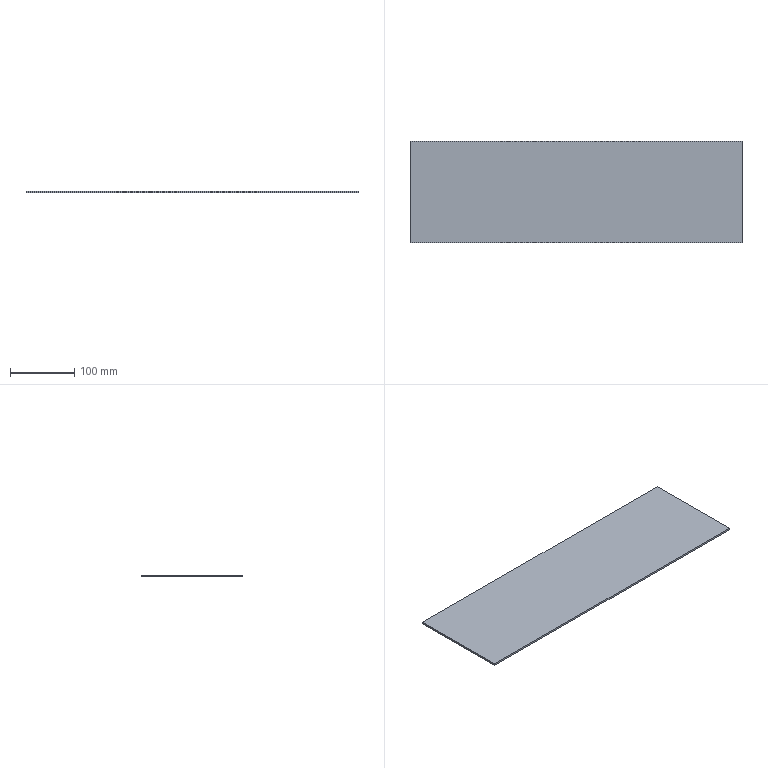Part | SolidWorks | features Extrusion 1 | 1 solid | 6 faces | box 515 x 158 x 3 mm | volume 244110 mm3 | plane 6
STEP:
#1=CARTESIAN_POINT('',(257.5,-79.,0.));
#2=VERTEX_POINT('',#1);
#3=CARTESIAN_POINT('',(257.5,79.,0.));
#4=VERTEX_POINT('',#3);
#5=CARTESIAN_POINT('',(257.5,79.,0.));
#6=DIRECTION('',(0.,1.,0.));
#7=VECTOR('',#6,1000.);
#8=LINE('',#5,#7);
#9=EDGE_CURVE('',#2,#4,#8,.T.);
#10=ORIENTED_EDGE('',*,*,#9,.T.);
#11=CARTESIAN_POINT('',(257.5,79.,3.));
#12=VERTEX_POINT('',#11);
#13=CARTESIAN_POINT('',(257.5,79.,3.));
#14=DIRECTION('',(0.,0.,-1.));
#15=VECTOR('',#14,1000.);
#16=LINE('',#13,#15);
#17=EDGE_CURVE('',#12,#4,#16,.T.);
#18=ORIENTED_EDGE('',*,*,#17,.F.);
#19=CARTESIAN_POINT('',(257.5,-79.,3.));
#20=VERTEX_POINT('',#19);
#21=CARTESIAN_POINT('',(257.5,79.,3.));
#22=DIRECTION('',(0.,1.,0.));
#23=VECTOR('',#22,1000.);
#24=LINE('',#21,#23);
#25=EDGE_CURVE('',#20,#12,#24,.T.);
#26=ORIENTED_EDGE('',*,*,#25,.F.);
#27=CARTESIAN_POINT('',(257.5,-79.,3.));
#28=DIRECTION('',(0.,0.,-1.));
#29=VECTOR('',#28,1000.);
#30=LINE('',#27,#29);
#31=EDGE_CURVE('',#20,#2,#30,.T.);
#32=ORIENTED_EDGE('',*,*,#31,.T.);
#33=EDGE_LOOP('',(#10,#18,#26,#32));
#34=FACE_OUTER_BOUND('',#33,.T.);
#35=CARTESIAN_POINT('',(257.5,79.,3.));
#36=DIRECTION('',(-1.,0.,0.));
#37=DIRECTION('',(0.,0.,1.));
#38=AXIS2_PLACEMENT_3D('',#35,#36,#37);
#39=PLANE('',#38);
#40=ADVANCED_FACE('',(#34),#39,.F.);
#41=CARTESIAN_POINT('',(-257.5,79.,0.));
#42=VERTEX_POINT('',#41);
#43=CARTESIAN_POINT('',(-257.5,79.,0.));
#44=DIRECTION('',(-1.,0.,0.));
#45=VECTOR('',#44,1000.);
#46=LINE('',#43,#45);
#47=EDGE_CURVE('',#4,#42,#46,.T.);
#48=ORIENTED_EDGE('',*,*,#47,.T.);
#49=CARTESIAN_POINT('',(-257.5,79.,3.));
#50=VERTEX_POINT('',#49);
#51=CARTESIAN_POINT('',(-257.5,79.,3.));
#52=DIRECTION('',(0.,0.,-1.));
#53=VECTOR('',#52,1000.);
#54=LINE('',#51,#53);
#55=EDGE_CURVE('',#50,#42,#54,.T.);
#56=ORIENTED_EDGE('',*,*,#55,.F.);
#57=CARTESIAN_POINT('',(-257.5,79.,3.));
#58=DIRECTION('',(-1.,0.,0.));
#59=VECTOR('',#58,1000.);
#60=LINE('',#57,#59);
#61=EDGE_CURVE('',#12,#50,#60,.T.);
#62=ORIENTED_EDGE('',*,*,#61,.F.);
#63=ORIENTED_EDGE('',*,*,#17,.T.);
#64=EDGE_LOOP('',(#48,#56,#62,#63));
#65=FACE_OUTER_BOUND('',#64,.T.);
#66=CARTESIAN_POINT('',(-257.5,79.,3.));
#67=DIRECTION('',(0.,-1.,0.));
#68=DIRECTION('',(0.,0.,-1.));
#69=AXIS2_PLACEMENT_3D('',#66,#67,#68);
#70=PLANE('',#69);
#71=ADVANCED_FACE('',(#65),#70,.F.);
#72=CARTESIAN_POINT('',(-257.5,-79.,0.));
#73=VERTEX_POINT('',#72);
#74=CARTESIAN_POINT('',(-257.5,79.,0.));
#75=DIRECTION('',(0.,-1.,0.));
#76=VECTOR('',#75,1000.);
#77=LINE('',#74,#76);
#78=EDGE_CURVE('',#42,#73,#77,.T.);
#79=ORIENTED_EDGE('',*,*,#78,.T.);
#80=CARTESIAN_POINT('',(-257.5,-79.,3.));
#81=VERTEX_POINT('',#80);
#82=CARTESIAN_POINT('',(-257.5,-79.,3.));
#83=DIRECTION('',(0.,0.,-1.));
#84=VECTOR('',#83,1000.);
#85=LINE('',#82,#84);
#86=EDGE_CURVE('',#81,#73,#85,.T.);
#87=ORIENTED_EDGE('',*,*,#86,.F.);
#88=CARTESIAN_POINT('',(-257.5,79.,3.));
#89=DIRECTION('',(0.,-1.,0.));
#90=VECTOR('',#89,1000.);
#91=LINE('',#88,#90);
#92=EDGE_CURVE('',#50,#81,#91,.T.);
#93=ORIENTED_EDGE('',*,*,#92,.F.);
#94=ORIENTED_EDGE('',*,*,#55,.T.);
#95=EDGE_LOOP('',(#79,#87,#93,#94));
#96=FACE_OUTER_BOUND('',#95,.T.);
#97=CARTESIAN_POINT('',(-257.5,79.,3.));
#98=DIRECTION('',(1.,0.,0.));
#99=DIRECTION('',(0.,0.,-1.));
#100=AXIS2_PLACEMENT_3D('',#97,#98,#99);
#101=PLANE('',#100);
#102=ADVANCED_FACE('',(#96),#101,.F.);
#103=CARTESIAN_POINT('',(-257.5,-79.,0.));
#104=DIRECTION('',(1.,0.,0.));
#105=VECTOR('',#104,1000.);
#106=LINE('',#103,#105);
#107=EDGE_CURVE('',#73,#2,#106,.T.);
#108=ORIENTED_EDGE('',*,*,#107,.T.);
#109=ORIENTED_EDGE('',*,*,#31,.F.);
#110=CARTESIAN_POINT('',(-257.5,-79.,3.));
#111=DIRECTION('',(1.,0.,0.));
#112=VECTOR('',#111,1000.);
#113=LINE('',#110,#112);
#114=EDGE_CURVE('',#81,#20,#113,.T.);
#115=ORIENTED_EDGE('',*,*,#114,.F.);
#116=ORIENTED_EDGE('',*,*,#86,.T.);
#117=EDGE_LOOP('',(#108,#109,#115,#116));
#118=FACE_OUTER_BOUND('',#117,.T.);
#119=CARTESIAN_POINT('',(-257.5,-79.,3.));
#120=DIRECTION('',(0.,1.,0.));
#121=DIRECTION('',(0.,0.,1.));
#122=AXIS2_PLACEMENT_3D('',#119,#120,#121);
#123=PLANE('',#122);
#124=ADVANCED_FACE('',(#118),#123,.F.);
#125=ORIENTED_EDGE('',*,*,#25,.T.);
#126=ORIENTED_EDGE('',*,*,#61,.T.);
#127=ORIENTED_EDGE('',*,*,#92,.T.);
#128=ORIENTED_EDGE('',*,*,#114,.T.);
#129=EDGE_LOOP('',(#125,#126,#127,#128));
#130=FACE_OUTER_BOUND('',#129,.T.);
#131=CARTESIAN_POINT('',(0.,0.,3.));
#132=DIRECTION('',(0.,0.,1.));
#133=DIRECTION('',(1.,0.,0.));
#134=AXIS2_PLACEMENT_3D('',#131,#132,#133);
#135=PLANE('',#134);
#136=ADVANCED_FACE('',(#130),#135,.T.);
#137=ORIENTED_EDGE('',*,*,#9,.F.);
#138=ORIENTED_EDGE('',*,*,#107,.F.);
#139=ORIENTED_EDGE('',*,*,#78,.F.);
#140=ORIENTED_EDGE('',*,*,#47,.F.);
#141=EDGE_LOOP('',(#137,#138,#139,#140));
#142=FACE_OUTER_BOUND('',#141,.T.);
#143=CARTESIAN_POINT('',(0.,0.,0.));
#144=DIRECTION('',(0.,0.,1.));
#145=DIRECTION('',(1.,0.,0.));
#146=AXIS2_PLACEMENT_3D('',#143,#144,#145);
#147=PLANE('',#146);
#148=ADVANCED_FACE('',(#142),#147,.F.);
#149=CLOSED_SHELL('',(#40,#71,#102,#124,#136,#148));
#150=MANIFOLD_SOLID_BREP('',#149);
#151=CARTESIAN_POINT('',(0.,0.,0.));
#152=DIRECTION('',(0.,0.,1.));
#153=DIRECTION('',(1.,0.,0.));
#154=AXIS2_PLACEMENT_3D('',#151,#152,#153);
#155=(LENGTH_UNIT()NAMED_UNIT(*)SI_UNIT(.MILLI.,.METRE.));
#156=UNCERTAINTY_MEASURE_WITH_UNIT(LENGTH_MEASURE(0.00001),#155,'','');
#157=(NAMED_UNIT(*)PLANE_ANGLE_UNIT()SI_UNIT($,.RADIAN.));
#158=(NAMED_UNIT(*)SI_UNIT($,.STERADIAN.)SOLID_ANGLE_UNIT());
#159=(GEOMETRIC_REPRESENTATION_CONTEXT(3)GLOBAL_UNCERTAINTY_ASSIGNED_CONTEXT((#156))GLOBAL_UNIT_ASSIGNED_CONTEXT((#155,#157,#158))REPRESENTATION_CONTEXT('',''));
#160=ADVANCED_BREP_SHAPE_REPRESENTATION('',(#150,#154),#159);